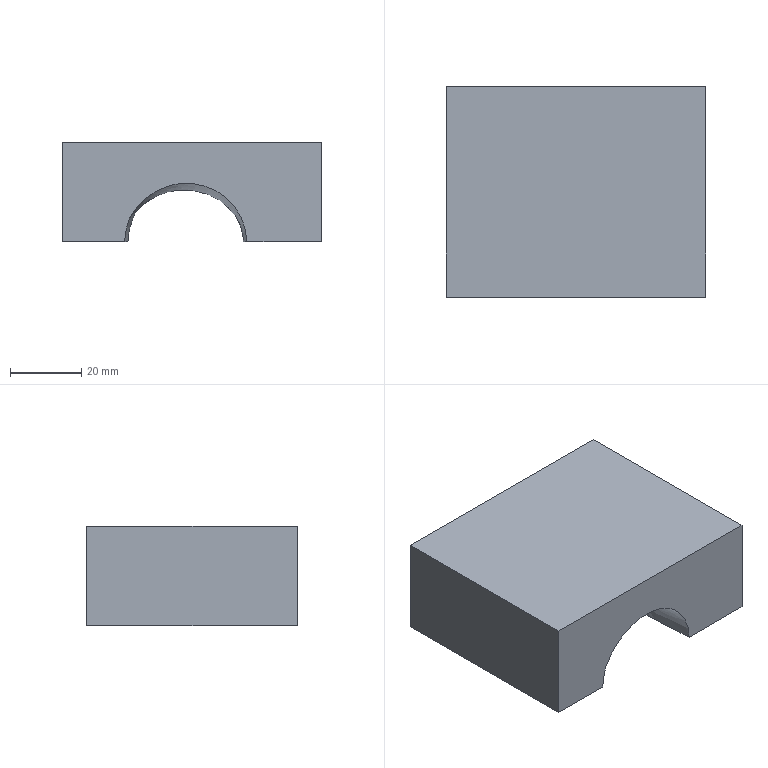NC program | NX | posted with a generic post | part box 72.744 x 59.015 x 27.972 mm
Lines 1006 to 1755 of 95982:
(ZLEVEL_PROFILE_COPY , TOOL : D6)
N1980 T16 M6
N1982 G54
N1984 G17 G0 G90 X-1.91 Y5.013 S9500 M3
N1986 G43 Z30. H16
N1988 Z-10.767
N1990 G94 G1 Z-13.767 F1000.
N1992 X-0.528 Y6.002
N1994 G3 X-0.28 Y6.548 R0.6
N1996 G2 X-0.429 Y9.381 R31.673 F2500.
N1998 X-0.097 Y12.574 R35.85
N2000 G1 X-0.091 Y12.841 Z-13.779
N2002 X-0.081 Y13.107 Z-13.791
N2004 X-0.138 Y13.385 Z-13.803
N2006 X-0.123 Y13.65 Z-13.816
N2008 X-0.108 Y13.916 Z-13.828
N2010 X-0.091 Y14.18 Z-13.84
N2012 X-0.073 Y14.445 Z-13.852
N2014 X-0.046 Y14.707 Z-13.864
N2016 G3 X-0.802 Y8.189 R29.106
N2018 X-0.377 Y4.736 R34.657
N2020 G1 X-0.411 Y4.471 Z-13.886
N2022 X-0.427 Y4.21 Z-13.908
N2024 X-0.462 Y3.946 Z-13.93
N2026 X-0.499 Y3.681 Z-13.952
N2028 G2 X-1.122 Y7.13 R36.802
N2030 X-0.76 Y12.795 R14.66
N2032 G1 X-0.717 Y12.958
N2034 X-0.512 Y13.72
N2036 G2 X0.069 Y16.291 R38.062
N2038 G1 X-0.01 Y16.55 Z-13.978
N2040 X-0.017 Y16.789 Z-14.005
N2042 X0.004 Y17.017 Z-14.031
N2044 X-0.352 Y15.939
N2046 X-0.479 Y15.343
N2048 G3 X-1.507 Y6.997 R19.989
N2050 X-0.537 Y2.644 R41.823
N2052 G1 X-0.56 Y2.42 Z-14.055
N2054 X-0.566 Y2.201 Z-14.079
N2056 X-0.624 Y1.966 Z-14.103
N2058 G2 X-1.857 Y6.997 R40.018
N2060 X-0.816 Y15.343 R19.684
N2062 G3 X0.117 Y17.995 R301.619
N2064 X0.004 Y18.584 R0.6
N2066 G1 X-1.132 Y19.897
N2068 Z-11.103
N2070 G0 Z30.
N2072 X-2.328 Y14.003
N2074 Z-10.767
N2076 G1 Z-13.767 F1000.
N2078 X-3.75 Y13.078
N2080 G3 X-4.022 Y12.543 R0.6
N2082 G2 X-4.284 Y6.876 R28.666 F2500.
N2084 G1 X-4.259 Y6.608 Z-13.781
N2086 X-4.269 Y6.346 Z-13.795
N2088 X-4.281 Y6.084 Z-13.809
N2090 X-4.294 Y5.823 Z-13.822
N2092 X-4.302 Y5.562 Z-13.836
N2094 X-4.29 Y5.296 Z-13.85
N2096 X-4.259 Y5.026 Z-13.864
N2098 G3 X-3.534 Y11.17 R28.408
N2100 X-3.968 Y14.949 R60.378
N2102 G1 X-3.905 Y15.239 Z-13.881
N2104 X-3.889 Y15.522 Z-13.899
N2106 X-3.881 Y15.804 Z-13.917
N2108 X-3.887 Y16.083 Z-13.934
N2110 X-3.888 Y16.363 Z-13.952
N2112 G2 X-3.363 Y13.12 R61.
N2114 X-4.233 Y3.858 R20.662
N2116 G1 X-4.19 Y3.578 Z-13.972
N2118 X-4.27 Y3.341 Z-13.992
N2120 X-4.279 Y3.079 Z-14.012
N2122 X-4.261 Y2.808 Z-14.031
N2124 G3 X-3.011 Y13.22 R21.101
N2126 X-3.75 Y17.133 R36.255
N2128 G1 X-3.708 Y17.441 Z-14.055
N2130 X-3.69 Y17.744 Z-14.079
N2132 X-3.729 Y18.031 Z-14.103
N2134 X-3.157 Y15.939
N2136 X-3.028 Y15.343
N2138 X-2.466 Y11.766
N2140 X-2.426 Y11.17
N2142 G2 X-4.076 Y2.539 R21.676
N2144 G3 X-4.295 Y2.015 R131.443
N2146 X-4.216 Y1.42 R0.6
N2148 G1 X-3.157 Y0.039
N2150 Z-11.103
N2152 G0 Z30.
N2154 X-1.052 Y20.692
N2156 Z-11.167
N2158 G1 Z-14.167 F1000.
N2160 X0.052 Y19.345
N2162 G2 X0.149 Y18.753 R0.6
N2164 X-0.376 Y17.387 R116.838 F2500.
N2166 G3 X-2.068 Y11.732 R35.835
N2168 G1 X-2.209 Y12.362
N2170 X-2.742 Y15.343
N2172 X-2.895 Y15.939
N2174 X-3.724 Y18.87
N2176 G2 X-3.576 Y19.452 R0.6
N2178 G1 X-2.368 Y20.693
N2180 Z-11.167
N2182 G0 Z30.
N2184 X-2.484 Y21.68
N2186 Z-11.23
N2188 G1 Z-14.23 F1000.
N2190 X-3.664 Y20.408
N2192 G3 X-3.798 Y19.823 R0.6
N2194 X-2.567 Y15.939 R274.089 F2500.
N2196 G1 X-2.196 Y14.151
N2198 X-1.758
N2200 G2 X-1.02 Y16.535 R13.546
N2202 G3 X0.288 Y19.692 R81.136
N2204 G1 X0.194 Y20.023 Z-14.263
N2206 X0.295 Y20.276 Z-14.295
N2208 G2 X-1.159 Y16.923 R71.26
N2210 G3 X-1.918 Y14.774 R11.953
N2212 G1 X-2.442 Y16.535
N2214 G2 X-3.704 Y20.28 R205.233
N2216 G1 X-3.604 Y20.507 Z-14.326
N2218 X-3.602 Y20.7 Z-14.358
N2220 G3 X-1.87 Y16.08 R133.71
N2222 X0.242 Y20.717 R68.25
N2224 G1 X0.138 Y20.953 Z-14.39
N2226 X0.163 Y21.134 Z-14.422
N2228 G2 X-0.814 Y19.011 R57.936
N2230 G1 X-1.7 Y17.181
N2232 X-1.865 Y16.983
N2234 G2 X-3.513 Y21.179 R115.641
N2236 G1 X-3.507 Y21.437 Z-14.455
N2238 X-3.456 Y21.711 Z-14.488
N2240 G3 X-1.824 Y17.772 R97.352
N2242 G1 X-1.7 Y17.906
N2244 X-0.516 Y20.312
N2246 G3 X0.096 Y21.599 R50.794
N2248 G1 X0.081 Y21.89 Z-14.52
N2250 X0.103 Y22.162 Z-14.553
N2252 G2 X-0.885 Y20.177 R46.933
N2254 G1 X-1.7 Y18.63
N2256 X-1.789 Y18.54
N2258 X-2.888 Y20.822
N2260 G2 X-3.511 Y22.4 R103.8
N2262 G1 X-3.507 Y22.611 Z-14.575
N2264 X-3.495 Y22.825 Z-14.597
N2266 X-3.522 Y23.024 Z-14.619
N2268 G3 X-2.888 Y21.453 R95.973
N2270 G1 X-1.755 Y19.308
N2272 G3 X0.15 Y22.77 R38.438
N2274 G1 X0.143 Y23.002 Z-14.641
N2276 X0.163 Y23.221 Z-14.663
N2278 X0.238 Y23.414 Z-14.685
N2280 G2 X-1.7 Y20.086 R28.965
N2282 X-2.888 Y22.086 R11.326
N2284 X-3.523 Y23.611 R84.847
N2286 G1 X-3.48 Y23.876 Z-14.717
N2288 X-3.494 Y24.118 Z-14.75
N2290 G3 X-2.972 Y22.902 R74.218
N2292 X-1.741 Y20.758 R11.608
N2294 X-0.512 Y22.43 R6.162
N2296 X0.243 Y23.955 R41.25
N2298 G1 X0.178 Y24.202 Z-14.782
N2300 X0.216 Y24.4 Z-14.814
N2302 G2 X-0.498 Y22.974 R39.444
N2304 X-1.7 Y21.349 R6.674
N2306 X-2.888 Y23.328 R12.916
N2308 X-3.422 Y24.516 R64.506
N2310 G1 X-3.401 Y24.756 Z-14.848
N2312 X-3.385 Y24.994 Z-14.881
N2314 G3 X-2.888 Y23.917 R59.21
N2316 X-1.7 Y21.917 R12.394
N2318 X-0.767 Y23.051 R4.084
N2320 G1 X-0.68 Y23.207
N2322 G3 X0.207 Y24.905 R35.835
N2324 G1 X0.19 Y25.194 Z-14.914
N2326 X0.255 Y25.443 Z-14.948
N2328 G2 X0.081 Y25.078 R38.756
N2330 X-1.684 Y22.513 R8.913
N2332 G1 X-2.888 Y24.462
N2334 G2 X-3.378 Y25.508 R56.473
N2336 G1 X-3.375 Y25.78 Z-14.982
N2338 X-3.386 Y26.045 Z-15.015
N2340 G3 X-2.888 Y24.993 R53.554
N2342 G1 X-1.661 Y23.093
N2344 G3 X0.081 Y25.583 R9.261
N2346 X0.281 Y26.002 R36.93
N2348 G1 X0.225 Y26.256 Z-15.049
N2350 X0.259 Y26.468 Z-15.083
N2352 G2 X0.081 Y26.098 R35.375
N2354 X-1.647 Y23.698 R7.866
N2356 G1 X-2.888 Y25.536
N2358 G2 X-3.401 Y26.602 R50.455
N2360 G1 X-3.378 Y26.869 Z-15.118
N2362 X-3.394 Y27.119 Z-15.152
N2364 G3 X-2.888 Y26.084 R47.643
N2366 G1 X-1.638 Y24.295
N2368 G3 X-0.092 Y26.266 R6.278
N2370 X0.265 Y27.001 R34.124
N2372 G1 X0.227 Y27.259 Z-15.186
N2374 X0.256 Y27.486 Z-15.219
N2376 G2 X-0.135 Y26.684 R33.135
N2378 X-1.618 Y24.851 R5.571
N2380 G1 X-1.7 Y24.91
N2382 X-2.888 Y26.619
N2384 G2 X-3.387 Y27.619 R44.08
N2386 G1 X-3.336 Y27.862 Z-15.254
N2388 X-3.35 Y28.073 Z-15.289
N2390 G3 X-2.888 Y27.173 R38.811
N2392 G1 X-1.7 Y25.456
N2394 X-1.593 Y25.387
N2396 G3 X-0.512 Y26.586 R3.729
N2398 G1 X-0.468 Y26.666
N2400 G3 X0.199 Y27.928 R27.656
N2402 G1 X0.175 Y28.192 Z-15.324
N2404 X0.189 Y28.436 Z-15.359
N2406 G2 X-0.512 Y27.112 R26.628
N2408 X-1.574 Y25.917 R3.697
N2410 X-3.345 Y28.557 R11.791
N2412 G1 X-3.308 Y28.803 Z-15.394
N2414 X-3.327 Y29.022 Z-15.429
N2416 G3 X-1.555 Y26.445 R11.412
N2418 X-0.628 Y27.439 R3.064
N2420 X0.198 Y28.976 R25.306
N2422 G1 X0.165 Y29.227 Z-15.464
N2424 X0.174 Y29.457 Z-15.499
N2426 G2 X-0.661 Y27.909 R24.255
N2428 X-1.556 Y26.986 R2.715
N2430 X-3.336 Y29.531 R11.534
N2432 G1 X-3.305 Y29.807 Z-15.534
N2434 X-3.348 Y30.046 Z-15.569
N2436 G3 X-1.536 Y27.514 R10.556
N2438 X-0.635 Y28.482 R3.029
N2440 X0.173 Y29.986 R23.112
N2442 G1 X0.162 Y30.278 Z-15.604
N2444 X0.186 Y30.553 Z-15.639
N2446 G2 X-0.663 Y28.961 R22.54
N2448 X-1.528 Y28.05 R2.759
N2450 X-3.366 Y30.583 R9.279
N2452 G1 X-3.322 Y30.874 Z-15.674
N2454 X-3.349 Y31.131 Z-15.709
N2456 X-3.324 Y31.075
N2458 G3 X-2. Y29.055 R7.522
N2460 G1 X-1.7 Y28.686
N2462 X-1.472 Y28.565
N2464 G3 X0.193 Y31.076 R7.26
N2466 G1 X0.278 Y31.291
N2468 X0.225 Y31.583 Z-15.744
N2470 X0.257 Y31.841 Z-15.779
N2472 X0.081 Y31.413
N2474 X-0.196 Y30.843
N2476 G2 X-1.479 Y29.077 R5.868
N2478 X-2.888 Y30.736 R5.339
N2480 G1 X-3.322 Y31.66
N2482 X-3.316 Y31.942 Z-15.815
N2484 X-3.345 Y32.206 Z-15.85
N2486 X-2.888 Y31.259
N2488 G3 X-1.507 Y29.59 R5.749
N2490 X-0.196 Y31.44 R4.925
N2492 G1 X0.171 Y32.268
N2494 X0.205 Y32.511 Z-15.867
N2496 X0.247 Y32.75 Z-15.885
N2498 X0.29 Y32.988 Z-15.902
N2500 X0.416 Y33.192 Z-15.92
N2502 G2 X-1.471 Y30.116 R11.06
N2504 G1 X-1.513 Y30.054
N2506 X-1.591
N2508 X-1.634 Y30.116
N2510 G2 X-3.456 Y32.827 R13.653
N2512 G1 X-3.39 Y33.097 Z-15.955
N2514 X-3.429 Y33.315 Z-15.99
N2516 G3 X-2.294 Y31.396 R17.007
N2518 G1 X-1.7 Y30.695
N2520 X-1.532 Y30.595
N2522 G3 X-0.483 Y32.036 R4.823
N2524 G1 X0.129 Y33.274
N2526 X0.139 Y33.528 Z-16.013
N2528 X0.164 Y33.773 Z-16.037
N2530 X0.241 Y33.997 Z-16.061
N2532 G2 X-1.546 Y31.108 R10.435
N2534 X-3.49 Y33.94 R9.663
N2536 G1 X-3.378 Y34.103 Z-16.096
N2538 X-3.364 Y34.221 Z-16.131
N2540 G3 X-1.566 Y31.631 R9.938
N2542 X0.028 Y34.108 R10.975
N2544 G1 X-0.093 Y34.152 Z-16.166
N2546 X-0.211 Y34.194 Z-16.201
N2548 G2 X-1.595 Y32.165 R8.452
N2550 X-3.135 Y34.293 R10.551
N2552 G1 X-2.904 Y34.366 Z-16.271
N2554 X-2.888 Y34.336
N2556 X-1.7 Y32.797
N2558 X-1.603 Y32.72
N2560 G3 X-0.456 Y34.283 R7.041
N2562 G1 X-0.58 Y34.338 Z-16.305
N2564 X-0.711 Y34.396 Z-16.34
N2566 G2 X-1.605 Y33.251 R5.087
N2568 G1 X-2.641 Y34.476
N2570 X-2.37 Y34.601 Z-16.409
N2572 X-1.7 Y33.818
N2574 X-1.615 Y33.769
N2576 X-1.578 Y33.796
N2578 X-0.943 Y34.538
N2580 X-1.069 Y34.64 Z-16.443
N2582 X-1.187 Y34.736 Z-16.477
N2584 X-1.622 Y34.28
N2586 X-1.7 Y34.325
N2588 X-2.106 Y34.765
N2590 G2 X-2.238 Y35.351 R0.6
N2592 G1 X-1.777 Y36.824
N2594 Z-13.477
N2596 G0 Z30.
N2598 X-1.85 Y-0.592
N2600 Z-11.167
N2602 G1 Z-14.167 F1000.
N2604 X-0.742 Y0.714
N2606 G3 X-0.634 Y1.305 R0.6
N2608 G2 X-1.706 Y4.612 R57.134 F2500.
N2610 X-2.235 Y7.798 R13.672
N2612 G1 X-2.365 Y6.997
N2614 X-3.667 Y2.823
N2616 X-4.076 Y1.906
N2618 G3 X-4.291 Y1.41 R113.632
N2620 G1 X-4.269 Y1.173 Z-14.188
N2622 X-4.276 Y0.948 Z-14.209
N2624 X-4.336 Y0.746 Z-14.23
N2626 G2 X-3.994 Y1.515 R106.581
N2628 G3 X-2.308 Y5.702 R56.717
N2630 X-0.685 Y0.718 R38.505
N2632 G1 X-0.693 Y0.465 Z-14.252
N2634 X-0.678 Y0.223 Z-14.273
N2636 X-0.601 Y0.005 Z-14.295
N2638 X-2.362 Y4.323
N2640 G3 X-4.341 Y0.143 R110.879
N2642 G1 X-4.303 Y-0.086 Z-14.316
N2644 X-4.306 Y-0.296 Z-14.337
N2646 X-4.381 Y-0.472 Z-14.358
N2648 G2 X-2.386 Y3.358 R67.131
N2650 G1 X-0.659 Y-0.456
N2652 X-0.674 Y-0.706 Z-14.379
N2654 X-0.663 Y-0.945 Z-14.401
N2656 X-0.568 Y-1.144 Z-14.422
N2658 G3 X-2.422 Y2.404 R82.154
N2660 X-4.397 Y-1.12 R20.206
N2662 G1 X-4.315 Y-1.384 Z-14.455
N2664 X-4.34 Y-1.596 Z-14.488
N2666 G2 X-4.204 Y-1.35 R44.604
N2668 X-2.433 Y1.631 R9.895
N2670 X-0.599 Y-1.647 R64.396
N2672 G1 X-0.674 Y-1.836 Z-14.52
N2674 X-0.693 Y-1.994 Z-14.553
N2676 G3 X-1.392 Y-0.754 R57.03
N2678 G1 X-1.7 Y-0.166
N2680 G3 X-2.514 Y0.952 R28.687
N2682 X-3.911 Y-1.35 R9.061
N2684 X-4.241 Y-1.923 R41.508
N2686 G1 X-4.265 Y-2.205 Z-14.586
N2688 X-4.314 Y-2.474 Z-14.619
N2690 G2 X-2.551 Y0.281 R30.369
N2692 G1 X-1.7 Y-0.754
N2694 G2 X-0.724 Y-2.421 R53.059
N2696 G1 X-0.76 Y-2.611 Z-14.652
N2698 X-0.795 Y-2.799 Z-14.685
N2700 G3 X-1.106 Y-2.273 R47.818
N2702 G1 X-2.294 Y-0.619
N2704 X-2.526 Y-0.344
N2706 G3 X-4.301 Y-2.92 R22.716
N2708 G1 X-4.331 Y-3.174 Z-14.706
N2710 X-4.37 Y-3.424 Z-14.728
N2712 X-4.474 Y-3.637 Z-14.75
N2714 G2 X-2.471 Y-0.982 R11.427
N2716 G1 X-2.294 Y-1.197
N2718 X-1.106 Y-2.729
N2720 G2 X-0.786 Y-3.261 R46.182
N2722 G1 X-0.789 Y-3.5 Z-14.782
N2724 X-0.773 Y-3.727 Z-14.814
N2726 G3 X-1.106 Y-3.182 R43.793
N2728 X-2.491 Y-1.533 R30.782
N2730 X-3.836 Y-3.138 R8.25
N2732 G1 X-3.936 Y-3.297
N2734 G3 X-4.21 Y-3.74 R33.689
N2736 G1 X-4.233 Y-3.995 Z-14.848
N2738 X-4.254 Y-4.252 Z-14.881
N2740 G2 X-3.482 Y-3.046 R32.593
N2742 G1 X-2.496 Y-2.1
N2744 G2 X-0.85 Y-4.076 R8.118
N2746 G1 X-0.785 Y-4.187
N2748 X-0.789 Y-4.453 Z-14.914
N2750 X-0.765 Y-4.702 Z-14.948
N2752 X-0.892 Y-4.484
N2754 G3 X-2.501 Y-2.622 R6.585
N2756 G1 X-3.482 Y-3.527
N2758 G3 X-4.27 Y-4.747 R31.402
N2760 G1 X-4.259 Y-4.988 Z-14.982
N2762 X-4.273 Y-5.213 Z-15.015
N2764 G2 X-3.482 Y-4.004 R30.186
N2766 G1 X-2.553 Y-3.138
N2768 X-2.478 Y-3.08
N2770 G2 X-1.198 Y-4.523 R9.547
N2772 X-0.79 Y-5.104 R27.632
N2774 G1 X-0.817 Y-5.366 Z-15.049
N2776 X-0.762 Y-5.571 Z-15.083
N2778 G3 X-1.106 Y-5.076 R29.624
N2780 G1 X-2.295 Y-3.734
N2782 X-2.477 Y-3.557
N2784 X-3.482 Y-4.491
N2786 G3 X-4.263 Y-5.638 R26.551
N2788 G1 X-4.217 Y-5.845 Z-15.118
N2790 Y-6.022 Z-15.152
N2792 G2 X-3.482 Y-4.982 R24.154
N2794 X-2.392 Y-4.163 R2.383
N2796 X-0.864 Y-5.868 R14.936
N2798 G1 X-0.949 Y-6.082 Z-15.186
N2800 X-0.922 Y-6.207 Z-15.219
N2802 G3 X-2.46 Y-4.567 R13.569
N2804 X-4.186 Y-6.354 R9.492
N2806 G1 X-4.098 Y-6.535 Z-15.254
N2808 X-4.082 Y-6.661 Z-15.289
N2810 G2 X-2.492 Y-5.107 R8.66
N2812 X-0.911 Y-6.632 R6.748
N2814 G1 X-0.979 Y-6.858 Z-15.324
N2816 X-0.935 Y-7.001 Z-15.359
N2818 G3 X-1.106 Y-6.768 R24.132
N2820 G1 X-2.294 Y-5.687
N2822 X-2.456 Y-5.621
N2824 G3 X-4.063 Y-7.053 R6.706
N2826 G1 X-4.041 Y-7.317 Z-15.394
N2828 X-4.083 Y-7.532 Z-15.429
N2830 X-4.076 Y-7.522
N2832 G2 X-2.546 Y-6.119 R4.625
N2834 G1 X-2.294 Y-6.18
N2836 X-1.106 Y-7.186
N2838 X-0.988 Y-7.35
N2840 X-0.996 Y-7.658 Z-15.464
N2842 X-0.902 Y-7.89 Z-15.499
N2844 X-1.037 Y-7.712
N2846 G3 X-2.552 Y-6.612 R3.203
N2848 X-3.924 Y-7.725 R3.093
N2850 G1 X-4.135 Y-8.033
N2852 X-4.105 Y-8.267 Z-15.534
N2854 X-4.132 Y-8.462 Z-15.569
N2856 X-3.963 Y-8.211
N2858 G2 X-2.562 Y-7.05 R3.208
N2860 X-1.106 Y-8.034 R2.938
N2862 G1 X-0.875 Y-8.343
N2864 X-0.912 Y-8.577 Z-15.604
N2866 X-0.88 Y-8.762 Z-15.639
N2868 G3 X-1.106 Y-8.459 R23.076
N2870 X-2.514 Y-7.458 R3.114
N2872 X-3.916 Y-8.579 R3.004
N2874 G1 X-4.133 Y-8.902
N2876 X-4.034 Y-9.06 Z-15.674
N2878 X-3.985 Y-9.183 Z-15.709
N2880 G2 X-3.482 Y-8.527 R16.635
N2882 X-2.504 Y-7.874 R1.901
N2884 X-0.934 Y-9.086 R4.674
N2886 G1 X-0.94 Y-9.376 Z-15.744
N2888 X-0.878 Y-9.61 Z-15.779
N2890 X-1.106 Y-9.313
N2892 G3 X-2.548 Y-8.304 R2.672
N2894 X-4.079 Y-9.703 R4.041
N2896 G1 X-4.044 Y-9.96 Z-15.815
N2898 X-4.089 Y-10.165 Z-15.85
N2900 X-4.076 Y-10.146
N2902 G2 X-2.532 Y-8.719 R3.979
N2904 X-1.223 Y-9.592 R2.579
N2906 X-0.892 Y-10.017 R20.347
N2908 G1 X-0.93 Y-10.218 Z-15.885
N2910 X-0.91 Y-10.372 Z-15.92
N2912 G3 X-2.417 Y-9.131 R5.523
N2914 X-3.409 Y-9.75 R1.74
N2916 G1 X-3.998 Y-10.493
N2918 X-3.99 Y-10.773 Z-15.955
N2920 X-4.054 Y-11.001 Z-15.99
N2922 X-4.035 Y-10.972
N2924 G2 X-2.477 Y-9.547 R4.294
N2926 X-0.897 Y-10.797 R5.102
N2928 G1 X-0.913 Y-11.07 Z-16.025
N2930 X-0.865 Y-11.289 Z-16.061
N2932 X-1.106 Y-10.987
N2934 G3 X-2.505 Y-9.984 R2.915
N2936 X-4.055 Y-11.45 R4.31
N2938 G1 X-4.008 Y-11.695 Z-16.096
N2940 X-4.049 Y-11.885 Z-16.131
N2942 G2 X-2.503 Y-10.418 R4.306
N2944 X-1.106 Y-11.408 R2.697
N2946 G1 X-0.859 Y-11.717
N2948 X-0.879 Y-11.942 Z-16.166
N2950 X-0.834 Y-12.114 Z-16.201
N2952 G3 X-2.451 Y-10.837 R4.665
N2954 G1 X-2.66 Y-10.908
N2956 X-3.482 Y-11.613
N2958 G3 X-3.921 Y-12.201 R13.613
N2960 X-3.975 Y-12.798 R0.6
N2962 G1 X-3.206 Y-14.462
N2964 Z-13.201
N2966 G0 Z30.
N2968 X-3.168 Y-14.92
N2970 Z-13.271
N2972 G1 Z-16.271 F1000.
N2974 X-4.022 Y-13.318
N2976 G2 X-4.002 Y-12.718 R0.6
N2978 G1 X-3.976 Y-12.677 F2500.
N2980 G2 X-2.485 Y-11.272 R3.963
N2982 X-1.232 Y-12.083 R2.381
N2984 G1 X-0.856 Y-12.551
N2986 X-0.845 Y-12.814 Z-16.305
N2988 X-0.806 Y-13.056 Z-16.34
N2990 G3 X-1.106 Y-12.651 R15.828
N2992 X-2.483 Y-11.697 R2.442
N2994 X-4.07 Y-13.269 R4.175
N2996 G1 X-4.007 Y-13.51 Z-16.374
N2998 X-4.02 Y-13.706 Z-16.409
N3000 G2 X-3.754 Y-13.273 R14.882
N3002 X-2.462 Y-12.111 R3.117
N3004 X-1.106 Y-13.061 R2.49
N3006 X-0.721 Y-13.593 R15.288
N3008 G1 X-0.73 Y-13.858 Z-16.443
N3010 X-0.688 Y-14.088 Z-16.477
N3012 G3 X-0.841 Y-13.869 R14.219
N3014 G1 X-1.106 Y-13.491
N3016 G3 X-2.418 Y-12.522 R2.836
N3018 G1 X-2.581 Y-12.579
N3020 X-3.414 Y-13.273
N3022 X-3.482 Y-13.347
N3024 G3 X-4.039 Y-14.241 R14.313
N3026 G1 X-4.002 Y-14.518 Z-16.511
N3028 X-4.042 Y-14.751 Z-16.545
N3030 G2 X-3.482 Y-13.831 R13.647
N3032 X-2.479 Y-12.955 R2.552
N3034 X-1.588 Y-13.388 R1.268
N3036 G1 X-1.106 Y-13.941
N3038 G2 X-0.646 Y-14.592 R13.782
N3040 G1 X-0.707 Y-14.802 Z-16.578
N3042 X-0.719 Y-14.979 Z-16.612
N3044 G3 X-1.764 Y-13.648 R12.716
N3046 X-2.979 Y-13.688 R0.794
N3048 X-3.962 Y-15.142 R12.28
N3050 G1 X-3.949 Y-15.421 Z-16.645
N3052 X-3.984 Y-15.673 Z-16.679
N3054 G2 X-3.482 Y-14.805 R12.45
N3056 X-2.4 Y-13.748 R2.937
N3058 X-1.7 Y-14.16 R1.491
N3060 G1 X-1.106 Y-14.841
N3062 G2 X-0.634 Y-15.524 R12.26
N3064 G1 X-0.653 Y-15.777 Z-16.712
N3066 X-0.625 Y-16. Z-16.745
N3068 G3 X-1.106 Y-15.288 R11.633
N3070 X-2.348 Y-14.171 R4.06
N3072 X-4.068 Y-16.254 R4.999
N3074 G1 X-4.115 Y-16.36
N3076 X-4.061 Y-16.622 Z-16.777
N3078 X-4.091 Y-16.848 Z-16.81
N3080 G2 X-2.425 Y-14.631 R5.733
N3082 G1 X-2.294 Y-14.599
N3084 X-1.7 Y-15.052
N3086 G2 X-0.63 Y-16.466 R10.434
N3088 G1 X-0.576 Y-16.714 Z-16.831
N3090 X-0.536 Y-16.971 Z-16.853
N3092 X-0.458 Y-17.205 Z-16.874
N3094 G3 X-1.13 Y-16.127 R10.23
N3096 X-2.319 Y-15.035 R3.892
N3098 X-3.796 Y-16.819 R4.826
N3100 X-4.055 Y-17.402 R10.709
N3102 G1 X-4.005 Y-17.629 Z-16.895
N3104 X-4.007 Y-17.836 Z-16.916
N3106 X-4.042 Y-18.03 Z-16.938
N3108 G2 X-3.806 Y-17.446 R10.097
N3110 G1 X-3.53 Y-16.85
N3112 G2 X-2.294 Y-15.479 R3.547
N3114 X-0.807 Y-17.088 R4.406
N3116 G1 X-0.512 Y-17.634
N3118 G2 X-0.408 Y-17.85 R10.288
N3120 G1 X-0.404 Y-18.099 Z-16.953
N3122 X-0.367 Y-18.333 Z-16.969
N3124 X-0.343 Y-18.573 Z-16.985
N3126 X-0.252 Y-18.786 Z-17.001
N3128 G3 X-0.579 Y-18.042 R9.103
N3130 G1 X-0.898 Y-17.446
N3132 G3 X-2.193 Y-15.908 R4.743
N3134 X-3.209 Y-16.85 R2.214
N3136 X-4.095 Y-18.987 R9.638
N3138 G1 X-4.053 Y-19.269 Z-17.017
N3140 X-4.066 Y-19.536 Z-17.033
N3142 X-4.048 Y-19.811 Z-17.049
N3144 X-4.098 Y-20.072 Z-17.064
N3146 G2 X-3.097 Y-17.247 R9.131
N3148 G1 X-2.888 Y-16.87
N3150 G2 X-2.294 Y-16.37 R2.753
N3152 X-1.233 Y-17.399 R3.148
N3154 X-0.129 Y-19.974 R8.848
N3156 X-0.293 Y-20.551 R0.6
N3158 G1 X-1.666 Y-21.882
N3160 Z-14.064
N3162 G0 Z30.
N3164 X-2.913 Y-27.537
N3166 Z-13.271
N3168 G1 Z-16.271 F1000.
N3170 X-3.454 Y-29.319
N3172 G3 X-3.318 Y-29.904 R0.6
N3174 X-2.782 Y-30.438 R11.15 F2500.
N3176 G2 X-1.944 Y-31.62 R2.558
N3178 X-1.11 Y-30.455 R3.132
N3180 G3 X-0.474 Y-29.802 R10.989
N3182 G1 X-0.499 Y-29.602 Z-16.305
N3184 X-0.461 Y-29.459 Z-16.34
N3186 G2 X-1.328 Y-30.29 R9.795
N3188 G1 X-1.919 Y-30.877
N3190 G3 X-2.538 Y-30.279 R2.079
N3192 G2 X-3.304 Y-29.569 R9.86
N3194 G1 X-3.27 Y-29.389 Z-16.374
N3196 X-3.285 Y-29.258 Z-16.409
N3198 G3 X-2.089 Y-30.205 R7.937
N3200 X-1.573 Y-30.092 R0.309
N3202 X-0.55 Y-29.188 R8.892
N3204 G1 X-0.583 Y-29.018 Z-16.443
N3206 X-0.576 Y-28.888 Z-16.477
N3208 G2 X-1.822 Y-29.848 R7.252
N3210 G1 X-2.035 Y-29.841
N3212 G2 X-3.21 Y-28.974 R7.113
N3214 G1 Y-28.767 Z-16.511
N3216 X-3.257 Y-28.612 Z-16.545
N3218 G3 X-2.066 Y-29.483 R6.221
N3220 G1 X-1.855 Y-29.5
N3222 X-1.106 Y-29.067
N3224 G3 X-0.475 Y-28.454 R7.85
N3226 G1 X-0.586 Y-28.231 Z-16.612
N3228 G2 X-1.7 Y-29.116 R6.427
N3230 X-2.779 Y-28.732 R1.506
N3232 X-3.294 Y-28.226 R8.129
N3234 G1 X-3.276 Y-27.926 Z-16.679
N3236 G3 X-3.012 Y-28.177 R5.996
N3238 G1 X-2.888 Y-28.295
N3240 X-2.264 Y-28.721
N3242 G3 X-1.642 Y-28.734 R0.57
N3244 X-0.628 Y-27.937 R5.804
N3246 G1 X-0.618 Y-27.732 Z-16.712
N3248 X-0.578 Y-27.558 Z-16.745
N3250 G2 X-1.7 Y-28.434 R5.144
N3252 X-2.888 Y-27.969 R1.596
N3254 X-3.314 Y-27.542 R6.435
N3256 G1 X-3.333 Y-27.32 Z-16.777
N3258 X-3.396 Y-27.136 Z-16.81
N3260 G3 X-1.976 Y-28.147 R3.877
N3262 X-0.315 Y-26.953 R3.364
N3264 G1 X-0.323 Y-26.72 Z-16.831
N3266 X-0.277 Y-26.526 Z-16.853
N3268 X-0.189 Y-26.354 Z-16.874
N3270 G2 X-1.836 Y-27.811 R3.266
N3272 X-3.65 Y-26.411 R2.685
N3274 G1 X-3.633 Y-26.133 Z-16.906
N3276 X-3.675 Y-25.885 Z-16.938
N3278 G3 X-3.482 Y-26.267 R10.097
N3280 G1 X-3.403 Y-26.389
N3282 X-2.901 Y-26.985
N3284 G3 X-1.7 Y-27.455 R1.304
N3286 X-0.078 Y-25.699 R3.817
N3288 G1 X-0.152 Y-25.48 Z-16.959
N3290 X-0.143 Y-25.296 Z-16.98
N3292 X-0.158 Y-25.101 Z-17.001
N3294 G2 X-0.512 Y-25.962 R9.103
N3296 X-1.977 Y-27.189 R2.087
N3298 X-3.095 Y-26.389 R1.781
N3300 G1 X-3.483 Y-25.793
N3302 G2 X-3.764 Y-25.158 R9.638
N3304 G1 X-3.791 Y-24.935 Z-17.017
N3306 X-3.806 Y-24.708 Z-17.033
N3308 X-3.816 Y-24.48 Z-17.049
N3310 X-3.862 Y-24.263 Z-17.064
N3312 G3 X-3.482 Y-25.307 R9.131
N3314 G1 X-3.064 Y-26.022
N3316 G3 X-1.987 Y-26.873 R1.886
N3318 X-0.911 Y-26.145 R1.498
N3320 G1 X-0.512 Y-25.46
N3322 G3 X-0.113 Y-24.223 R8.848
N3324 X-0.281 Y-23.647 R0.6
N3326 G1 X-1.665 Y-22.326
N3328 Z-14.064
N3330 G0 Z30.
N3332 X-1.991 Y-23.387
N3334 Z-14.128
N3336 G1 Z-17.128 F1000.
N3338 X-2.564 Y-25.793
N3340 G2 X-3.085 Y-25.495 R0.6
N3342 G1 X-3.258 Y-25.196 F2500.
N3344 G2 X-3.482 Y-18.724 R8.61
N3346 G1 X-3.334 Y-18.322
N3348 G2 X-2.294 Y-16.823 R3.641
N3350 G1 X-2.227 Y-16.827
N3352 X-1.556 Y-17.446
N3354 G2 X-0.512 Y-24.859 R8.443
N3356 G1 X-0.655 Y-25.196
N3358 G2 X-1.87 Y-26.547 R2.524
N3360 X-2.911 Y-25.793 R1.511
N3362 G1 X-3.085 Y-25.495
N3364 X-3.156 Y-25.223 Z-17.136
N3366 X-3.257 Y-24.966 Z-17.145
N3368 X-3.333 Y-24.695 Z-17.153
N3370 X-3.399 Y-24.42 Z-17.161
N3372 X-3.464 Y-24.145 Z-17.169
N3374 X-3.523 Y-23.869 Z-17.177
N3376 X-3.563 Y-23.589 Z-17.185
N3378 X-3.658 Y-23.324 Z-17.193
N3380 G3 X-2.427 Y-25.947 R6.562
N3382 X-1.461 Y-25.935 R0.606
N3384 X-0.512 Y-20.559 R6.107
N3386 X-2.247 Y-17.258 R5.438
N3388 X-3.64 Y-20.427 R5.56
N3390 X-3.658 Y-23.324 R6.562
N3392 G1 X-3.506 Y-23.295 Z-17.225
N3394 X-3.397 Y-23.275 Z-17.257
N3396 G2 X-3.482 Y-22.538 R5.218
N3398 X-2.218 Y-17.751 R6.604
N3400 X-0.604 Y-21.619 R6.055
N3402 X-1.7 Y-25.728 R5.187
N3404 X-2.056 Y-25.793 R0.296
N3406 G1 X-2.294 Y-25.626
N3408 G2 X-3.397 Y-23.275 R5.218
N3410 G1 X-3.245 Y-23.242 Z-17.29
N3412 X-3.124 Y-23.216 Z-17.322
N3414 G3 X-2.654 Y-24.6 R6.376
N3416 X-1.941 Y-25.469 R2.701
N3418 X-0.938 Y-23.503 R4.101
N3420 X-2.189 Y-18.322 R6.309
N3422 X-3.124 Y-23.216 R6.376
N3424 G1 X-2.976 Y-23.182 Z-17.355
N3426 X-2.842 Y-23.152 Z-17.388
N3428 G2 X-2.169 Y-18.958 R5.705
N3430 X-1.403 Y-24.052 R5.666
N3432 X-1.971 Y-24.939 R2.159
N3434 G1 X-2.294 Y-24.61
N3436 G2 X-2.842 Y-23.152 R5.705
N3438 X-2.664 Y-22.579 R0.6
N3440 G1 Z-14.388
N3442 G0 Z30.
N3444 X-1.453 Y-22.073
N3446 Z-14.388
N3448 G1 Z-17.454 F1000.
N3450 G3 X-2.145 Y-19.715 R5.043 F2500.
N3452 X-1.958 Y-24.478 R5.176
N3454 X-1.453 Y-22.073 R5.043
N3456 G1 X-1.627 Y-22.098 Z-17.488
N3458 X-1.8 Y-22.122 Z-17.521
N3460 G2 X-1.985 Y-23.595 R4.556
N3462 X-2.098 Y-20.669 R4.673
N3464 X-1.8 Y-22.122 R4.556
N3466 X-2.08 Y-22.653 R0.6
N3468 G1 Z-14.521
N3470 G0 Z30.
N3472 M5